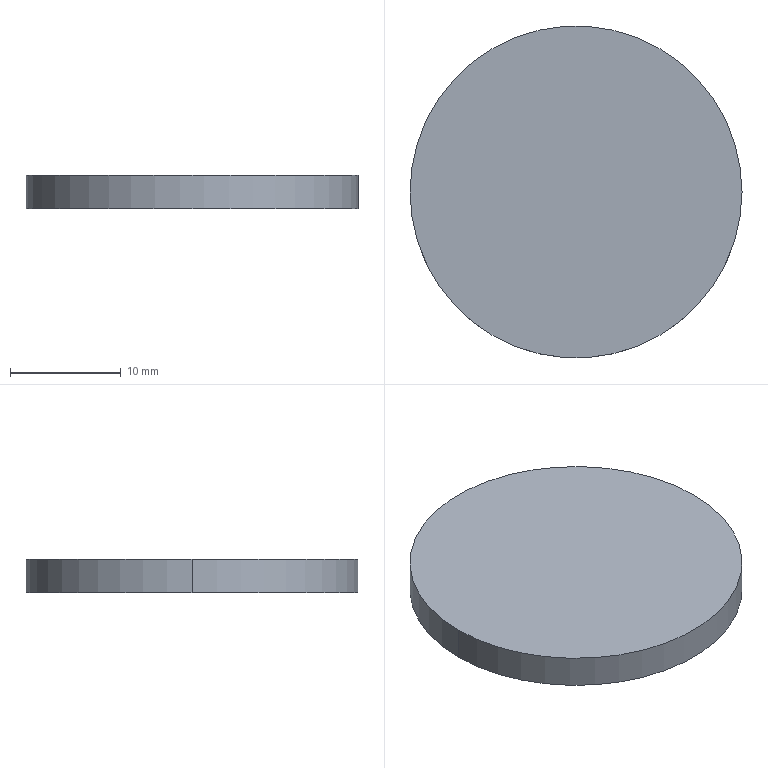Part | STEP file | TCHK-2D-D30-BB-30X3.stp.STEP | 1 solid | 4 faces | box 30 x 30 x 3 mm | volume 2121 mm3 | plane 2 | cylinder 2 | commonest cylinder face diameters 30 x2
STEP:
#1=CARTESIAN_POINT('',(-15.,0.,0.));
#2=VERTEX_POINT('',#1);
#3=CARTESIAN_POINT('',(15.,0.,0.));
#4=VERTEX_POINT('',#3);
#5=CARTESIAN_POINT('',(0.,0.,0.));
#6=DIRECTION('',(0.,0.,1.));
#7=DIRECTION('',(-1.,0.,0.));
#8=AXIS2_PLACEMENT_3D('',#5,#6,#7);
#9=CIRCLE('',#8,15.);
#10=EDGE_CURVE('',#2,#4,#9,.T.);
#11=ORIENTED_EDGE('',*,*,#10,.F.);
#12=CARTESIAN_POINT('',(0.,0.,0.));
#13=DIRECTION('',(0.,0.,1.));
#14=DIRECTION('',(1.,0.,0.));
#15=AXIS2_PLACEMENT_3D('',#12,#13,#14);
#16=CIRCLE('',#15,15.);
#17=EDGE_CURVE('',#4,#2,#16,.T.);
#18=ORIENTED_EDGE('',*,*,#17,.F.);
#19=EDGE_LOOP('',(#11,#18));
#20=FACE_OUTER_BOUND('',#19,.T.);
#21=CARTESIAN_POINT('',(0.,0.,0.));
#22=DIRECTION('',(0.,0.,1.));
#23=DIRECTION('',(1.,0.,0.));
#24=AXIS2_PLACEMENT_3D('',#21,#22,#23);
#25=PLANE('',#24);
#26=ADVANCED_FACE('',(#20),#25,.F.);
#27=CARTESIAN_POINT('',(-15.,0.,3.));
#28=VERTEX_POINT('',#27);
#29=CARTESIAN_POINT('',(-15.,0.,0.));
#30=DIRECTION('',(0.,0.,1.));
#31=VECTOR('',#30,1000.);
#32=LINE('',#29,#31);
#33=EDGE_CURVE('',#2,#28,#32,.T.);
#34=ORIENTED_EDGE('',*,*,#33,.T.);
#35=CARTESIAN_POINT('',(15.,0.,3.));
#36=VERTEX_POINT('',#35);
#37=CARTESIAN_POINT('',(0.,0.,3.));
#38=DIRECTION('',(0.,0.,1.));
#39=DIRECTION('',(1.,0.,0.));
#40=AXIS2_PLACEMENT_3D('',#37,#38,#39);
#41=CIRCLE('',#40,15.);
#42=EDGE_CURVE('',#36,#28,#41,.T.);
#43=ORIENTED_EDGE('',*,*,#42,.F.);
#44=CARTESIAN_POINT('',(15.,0.,0.));
#45=DIRECTION('',(0.,0.,1.));
#46=VECTOR('',#45,1000.);
#47=LINE('',#44,#46);
#48=EDGE_CURVE('',#4,#36,#47,.T.);
#49=ORIENTED_EDGE('',*,*,#48,.F.);
#50=ORIENTED_EDGE('',*,*,#17,.T.);
#51=EDGE_LOOP('',(#34,#43,#49,#50));
#52=FACE_OUTER_BOUND('',#51,.T.);
#53=CARTESIAN_POINT('',(0.,0.,0.));
#54=DIRECTION('',(0.,0.,1.));
#55=DIRECTION('',(1.,0.,0.));
#56=AXIS2_PLACEMENT_3D('',#53,#54,#55);
#57=CYLINDRICAL_SURFACE('',#56,15.);
#58=ADVANCED_FACE('',(#52),#57,.T.);
#59=ORIENTED_EDGE('',*,*,#48,.T.);
#60=CARTESIAN_POINT('',(0.,0.,3.));
#61=DIRECTION('',(0.,0.,1.));
#62=DIRECTION('',(-1.,0.,0.));
#63=AXIS2_PLACEMENT_3D('',#60,#61,#62);
#64=CIRCLE('',#63,15.);
#65=EDGE_CURVE('',#28,#36,#64,.T.);
#66=ORIENTED_EDGE('',*,*,#65,.F.);
#67=ORIENTED_EDGE('',*,*,#33,.F.);
#68=ORIENTED_EDGE('',*,*,#10,.T.);
#69=EDGE_LOOP('',(#59,#66,#67,#68));
#70=FACE_OUTER_BOUND('',#69,.T.);
#71=CARTESIAN_POINT('',(0.,0.,0.));
#72=DIRECTION('',(0.,0.,1.));
#73=DIRECTION('',(1.,0.,0.));
#74=AXIS2_PLACEMENT_3D('',#71,#72,#73);
#75=CYLINDRICAL_SURFACE('',#74,15.);
#76=ADVANCED_FACE('',(#70),#75,.T.);
#77=ORIENTED_EDGE('',*,*,#65,.T.);
#78=ORIENTED_EDGE('',*,*,#42,.T.);
#79=EDGE_LOOP('',(#77,#78));
#80=FACE_OUTER_BOUND('',#79,.T.);
#81=CARTESIAN_POINT('',(0.,0.,3.));
#82=DIRECTION('',(0.,0.,1.));
#83=DIRECTION('',(1.,0.,0.));
#84=AXIS2_PLACEMENT_3D('',#81,#82,#83);
#85=PLANE('',#84);
#86=ADVANCED_FACE('',(#80),#85,.T.);
#87=CLOSED_SHELL('',(#26,#58,#76,#86));
#88=MANIFOLD_SOLID_BREP('',#87);
#89=CARTESIAN_POINT('',(0.,0.,0.));
#90=DIRECTION('',(0.,0.,1.));
#91=DIRECTION('',(1.,0.,0.));
#92=AXIS2_PLACEMENT_3D('',#89,#90,#91);
#93=(LENGTH_UNIT()NAMED_UNIT(*)SI_UNIT(.MILLI.,.METRE.));
#94=UNCERTAINTY_MEASURE_WITH_UNIT(LENGTH_MEASURE(0.00001),#93,'','');
#95=(NAMED_UNIT(*)PLANE_ANGLE_UNIT()SI_UNIT($,.RADIAN.));
#96=(NAMED_UNIT(*)SI_UNIT($,.STERADIAN.)SOLID_ANGLE_UNIT());
#97=(GEOMETRIC_REPRESENTATION_CONTEXT(3)GLOBAL_UNCERTAINTY_ASSIGNED_CONTEXT((#94))GLOBAL_UNIT_ASSIGNED_CONTEXT((#93,#95,#96))REPRESENTATION_CONTEXT('',''));
#98=ADVANCED_BREP_SHAPE_REPRESENTATION('',(#88,#92),#97);